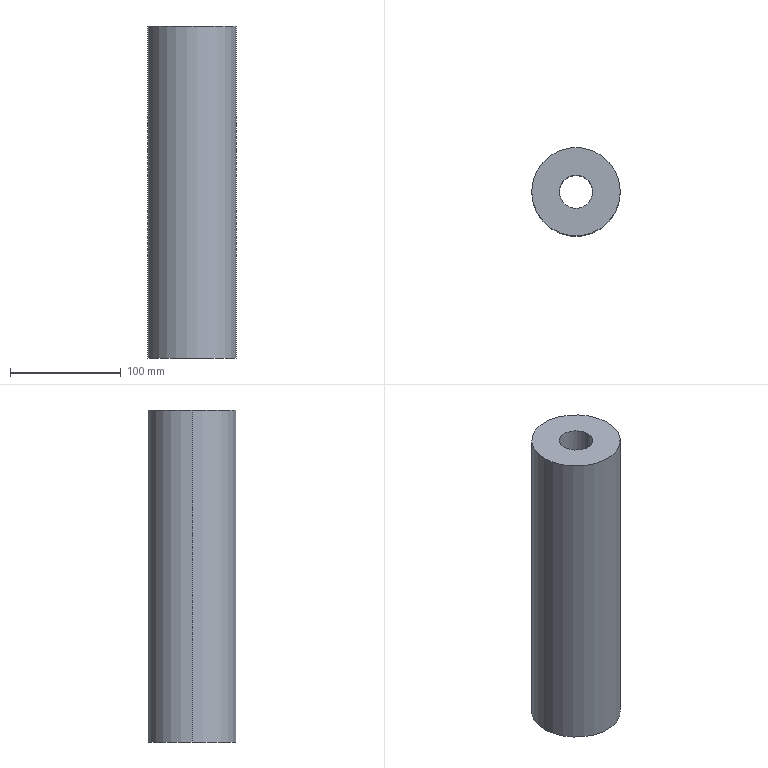Part | STEP file | Shaft for belt1V11 | 1 solid | 6 faces | box 80 x 80 x 300 mm | volume 1295907 mm3 | cylinder 4 | plane 2 | commonest cylinder face diameters 30 x2 80 x2
STEP:
#1=CARTESIAN_POINT('',(0.,0.,0.));
#2=DIRECTION('',(0.,0.,1.));
#3=DIRECTION('',(1.,0.,0.));
#4=AXIS2_PLACEMENT_3D('',#1,#2,#3);
#5=CARTESIAN_POINT('',(-15.,0.,300.));
#6=VERTEX_POINT('',#5);
#7=CARTESIAN_POINT('',(-15.,0.,0.));
#8=VERTEX_POINT('',#7);
#9=CARTESIAN_POINT('',(-15.,0.,300.));
#10=DIRECTION('',(0.,0.,-1.));
#11=VECTOR('',#10,1.);
#12=LINE('',#9,#11);
#13=CARTESIAN_POINT('',(0.,0.,300.));
#14=DIRECTION('',(0.,0.,-1.));
#15=DIRECTION('',(-1.,0.,0.));
#16=AXIS2_PLACEMENT_3D('',#13,#14,#15);
#17=CYLINDRICAL_SURFACE('',#16,15.);
#18=CARTESIAN_POINT('',(6.283,0.));
#19=DIRECTION('',(0.,1.));
#20=VECTOR('',#19,1.);
#21=LINE('',#18,#20);
#22=(GEOMETRIC_REPRESENTATION_CONTEXT(2)PARAMETRIC_REPRESENTATION_CONTEXT()REPRESENTATION_CONTEXT('',''));
#23=DEFINITIONAL_REPRESENTATION('',(#21),#22);
#24=PCURVE('',#17,#23);
#25=CARTESIAN_POINT('',(0.,0.,300.));
#26=DIRECTION('',(0.,0.,-1.));
#27=DIRECTION('',(-1.,0.,0.));
#28=AXIS2_PLACEMENT_3D('',#25,#26,#27);
#29=CYLINDRICAL_SURFACE('',#28,15.);
#30=CARTESIAN_POINT('',(0.,0.));
#31=DIRECTION('',(0.,1.));
#32=VECTOR('',#31,1.);
#33=LINE('',#30,#32);
#34=(GEOMETRIC_REPRESENTATION_CONTEXT(2)PARAMETRIC_REPRESENTATION_CONTEXT()REPRESENTATION_CONTEXT('',''));
#35=DEFINITIONAL_REPRESENTATION('',(#33),#34);
#36=PCURVE('',#29,#35);
#37=SURFACE_CURVE('',#12,(#24,#36),.PCURVE_S1.);
#38=EDGE_CURVE('',#6,#8,#37,.T.);
#39=ORIENTED_EDGE('',*,*,#38,.T.);
#40=CARTESIAN_POINT('',(15.,0.,0.));
#41=VERTEX_POINT('',#40);
#42=CARTESIAN_POINT('',(0.,0.,0.));
#43=DIRECTION('',(0.,0.,1.));
#44=DIRECTION('',(1.,0.,0.));
#45=AXIS2_PLACEMENT_3D('',#42,#43,#44);
#46=CIRCLE('',#45,15.);
#47=CARTESIAN_POINT('',(9.425,300.));
#48=DIRECTION('',(-1.,0.));
#49=VECTOR('',#48,1.);
#50=LINE('',#47,#49);
#51=(GEOMETRIC_REPRESENTATION_CONTEXT(2)PARAMETRIC_REPRESENTATION_CONTEXT()REPRESENTATION_CONTEXT('',''));
#52=DEFINITIONAL_REPRESENTATION('',(#50),#51);
#53=PCURVE('',#17,#52);
#54=CARTESIAN_POINT('',(0.,0.,0.));
#55=DIRECTION('',(0.,0.,1.));
#56=DIRECTION('',(1.,0.,0.));
#57=AXIS2_PLACEMENT_3D('',#54,#55,#56);
#58=PLANE('',#57);
#59=CARTESIAN_POINT('',(0.,0.));
#60=DIRECTION('',(1.,0.));
#61=AXIS2_PLACEMENT_2D('',#59,#60);
#62=CIRCLE('',#61,15.);
#63=(GEOMETRIC_REPRESENTATION_CONTEXT(2)PARAMETRIC_REPRESENTATION_CONTEXT()REPRESENTATION_CONTEXT('',''));
#64=DEFINITIONAL_REPRESENTATION('',(#62),#63);
#65=PCURVE('',#58,#64);
#66=SURFACE_CURVE('',#46,(#53,#65),.PCURVE_S1.);
#67=EDGE_CURVE('',#8,#41,#66,.T.);
#68=ORIENTED_EDGE('',*,*,#67,.T.);
#69=CARTESIAN_POINT('',(15.,0.,300.));
#70=VERTEX_POINT('',#69);
#71=CARTESIAN_POINT('',(15.,0.,300.));
#72=DIRECTION('',(0.,0.,-1.));
#73=VECTOR('',#72,1.);
#74=LINE('',#71,#73);
#75=CARTESIAN_POINT('',(3.142,0.));
#76=DIRECTION('',(0.,1.));
#77=VECTOR('',#76,1.);
#78=LINE('',#75,#77);
#79=(GEOMETRIC_REPRESENTATION_CONTEXT(2)PARAMETRIC_REPRESENTATION_CONTEXT()REPRESENTATION_CONTEXT('',''));
#80=DEFINITIONAL_REPRESENTATION('',(#78),#79);
#81=PCURVE('',#17,#80);
#82=CARTESIAN_POINT('',(3.142,0.));
#83=DIRECTION('',(0.,1.));
#84=VECTOR('',#83,1.);
#85=LINE('',#82,#84);
#86=(GEOMETRIC_REPRESENTATION_CONTEXT(2)PARAMETRIC_REPRESENTATION_CONTEXT()REPRESENTATION_CONTEXT('',''));
#87=DEFINITIONAL_REPRESENTATION('',(#85),#86);
#88=PCURVE('',#29,#87);
#89=SURFACE_CURVE('',#74,(#81,#88),.PCURVE_S1.);
#90=EDGE_CURVE('',#70,#41,#89,.T.);
#91=ORIENTED_EDGE('',*,*,#90,.F.);
#92=CARTESIAN_POINT('',(0.,0.,300.));
#93=DIRECTION('',(0.,0.,1.));
#94=DIRECTION('',(1.,0.,0.));
#95=AXIS2_PLACEMENT_3D('',#92,#93,#94);
#96=CIRCLE('',#95,15.);
#97=CARTESIAN_POINT('',(9.425,0.));
#98=DIRECTION('',(-1.,0.));
#99=VECTOR('',#98,1.);
#100=LINE('',#97,#99);
#101=(GEOMETRIC_REPRESENTATION_CONTEXT(2)PARAMETRIC_REPRESENTATION_CONTEXT()REPRESENTATION_CONTEXT('',''));
#102=DEFINITIONAL_REPRESENTATION('',(#100),#101);
#103=PCURVE('',#17,#102);
#104=CARTESIAN_POINT('',(0.,0.,300.));
#105=DIRECTION('',(0.,0.,1.));
#106=DIRECTION('',(1.,0.,0.));
#107=AXIS2_PLACEMENT_3D('',#104,#105,#106);
#108=PLANE('',#107);
#109=CARTESIAN_POINT('',(0.,0.));
#110=DIRECTION('',(1.,0.));
#111=AXIS2_PLACEMENT_2D('',#109,#110);
#112=CIRCLE('',#111,15.);
#113=(GEOMETRIC_REPRESENTATION_CONTEXT(2)PARAMETRIC_REPRESENTATION_CONTEXT()REPRESENTATION_CONTEXT('',''));
#114=DEFINITIONAL_REPRESENTATION('',(#112),#113);
#115=PCURVE('',#108,#114);
#116=SURFACE_CURVE('',#96,(#103,#115),.PCURVE_S1.);
#117=EDGE_CURVE('',#6,#70,#116,.T.);
#118=ORIENTED_EDGE('',*,*,#117,.F.);
#119=EDGE_LOOP('',(#39,#68,#91,#118));
#120=FACE_BOUND('',#119,.F.);
#121=ADVANCED_FACE('',(#120),#17,.F.);
#122=CARTESIAN_POINT('',(40.,0.,300.));
#123=VERTEX_POINT('',#122);
#124=CARTESIAN_POINT('',(-40.,0.,300.));
#125=VERTEX_POINT('',#124);
#126=CARTESIAN_POINT('',(0.,0.,300.));
#127=DIRECTION('',(0.,0.,1.));
#128=DIRECTION('',(1.,0.,0.));
#129=AXIS2_PLACEMENT_3D('',#126,#127,#128);
#130=CIRCLE('',#129,40.);
#131=CARTESIAN_POINT('',(0.,0.,300.));
#132=DIRECTION('',(0.,0.,-1.));
#133=DIRECTION('',(-1.,0.,0.));
#134=AXIS2_PLACEMENT_3D('',#131,#132,#133);
#135=CYLINDRICAL_SURFACE('',#134,40.);
#136=CARTESIAN_POINT('',(3.142,0.));
#137=DIRECTION('',(-1.,0.));
#138=VECTOR('',#137,1.);
#139=LINE('',#136,#138);
#140=(GEOMETRIC_REPRESENTATION_CONTEXT(2)PARAMETRIC_REPRESENTATION_CONTEXT()REPRESENTATION_CONTEXT('',''));
#141=DEFINITIONAL_REPRESENTATION('',(#139),#140);
#142=PCURVE('',#135,#141);
#143=CARTESIAN_POINT('',(0.,0.));
#144=DIRECTION('',(1.,0.));
#145=AXIS2_PLACEMENT_2D('',#143,#144);
#146=CIRCLE('',#145,40.);
#147=(GEOMETRIC_REPRESENTATION_CONTEXT(2)PARAMETRIC_REPRESENTATION_CONTEXT()REPRESENTATION_CONTEXT('',''));
#148=DEFINITIONAL_REPRESENTATION('',(#146),#147);
#149=PCURVE('',#108,#148);
#150=SURFACE_CURVE('',#130,(#142,#149),.PCURVE_S1.);
#151=EDGE_CURVE('',#123,#125,#150,.T.);
#152=ORIENTED_EDGE('',*,*,#151,.F.);
#153=CARTESIAN_POINT('',(40.,0.,0.));
#154=VERTEX_POINT('',#153);
#155=CARTESIAN_POINT('',(40.,0.,300.));
#156=DIRECTION('',(0.,0.,-1.));
#157=VECTOR('',#156,1.);
#158=LINE('',#155,#157);
#159=CARTESIAN_POINT('',(3.142,0.));
#160=DIRECTION('',(0.,1.));
#161=VECTOR('',#160,1.);
#162=LINE('',#159,#161);
#163=(GEOMETRIC_REPRESENTATION_CONTEXT(2)PARAMETRIC_REPRESENTATION_CONTEXT()REPRESENTATION_CONTEXT('',''));
#164=DEFINITIONAL_REPRESENTATION('',(#162),#163);
#165=PCURVE('',#135,#164);
#166=CARTESIAN_POINT('',(0.,0.,300.));
#167=DIRECTION('',(0.,0.,-1.));
#168=DIRECTION('',(-1.,0.,0.));
#169=AXIS2_PLACEMENT_3D('',#166,#167,#168);
#170=CYLINDRICAL_SURFACE('',#169,40.);
#171=CARTESIAN_POINT('',(3.142,0.));
#172=DIRECTION('',(0.,1.));
#173=VECTOR('',#172,1.);
#174=LINE('',#171,#173);
#175=(GEOMETRIC_REPRESENTATION_CONTEXT(2)PARAMETRIC_REPRESENTATION_CONTEXT()REPRESENTATION_CONTEXT('',''));
#176=DEFINITIONAL_REPRESENTATION('',(#174),#175);
#177=PCURVE('',#170,#176);
#178=SURFACE_CURVE('',#158,(#165,#177),.PCURVE_S1.);
#179=EDGE_CURVE('',#123,#154,#178,.T.);
#180=ORIENTED_EDGE('',*,*,#179,.T.);
#181=CARTESIAN_POINT('',(-40.,0.,0.));
#182=VERTEX_POINT('',#181);
#183=CARTESIAN_POINT('',(0.,0.,0.));
#184=DIRECTION('',(0.,0.,1.));
#185=DIRECTION('',(1.,0.,0.));
#186=AXIS2_PLACEMENT_3D('',#183,#184,#185);
#187=CIRCLE('',#186,40.);
#188=CARTESIAN_POINT('',(3.142,300.));
#189=DIRECTION('',(-1.,0.));
#190=VECTOR('',#189,1.);
#191=LINE('',#188,#190);
#192=(GEOMETRIC_REPRESENTATION_CONTEXT(2)PARAMETRIC_REPRESENTATION_CONTEXT()REPRESENTATION_CONTEXT('',''));
#193=DEFINITIONAL_REPRESENTATION('',(#191),#192);
#194=PCURVE('',#135,#193);
#195=CARTESIAN_POINT('',(0.,0.));
#196=DIRECTION('',(1.,0.));
#197=AXIS2_PLACEMENT_2D('',#195,#196);
#198=CIRCLE('',#197,40.);
#199=(GEOMETRIC_REPRESENTATION_CONTEXT(2)PARAMETRIC_REPRESENTATION_CONTEXT()REPRESENTATION_CONTEXT('',''));
#200=DEFINITIONAL_REPRESENTATION('',(#198),#199);
#201=PCURVE('',#58,#200);
#202=SURFACE_CURVE('',#187,(#194,#201),.PCURVE_S1.);
#203=EDGE_CURVE('',#154,#182,#202,.T.);
#204=ORIENTED_EDGE('',*,*,#203,.T.);
#205=CARTESIAN_POINT('',(-40.,0.,300.));
#206=DIRECTION('',(0.,0.,-1.));
#207=VECTOR('',#206,1.);
#208=LINE('',#205,#207);
#209=CARTESIAN_POINT('',(0.,0.));
#210=DIRECTION('',(0.,1.));
#211=VECTOR('',#210,1.);
#212=LINE('',#209,#211);
#213=(GEOMETRIC_REPRESENTATION_CONTEXT(2)PARAMETRIC_REPRESENTATION_CONTEXT()REPRESENTATION_CONTEXT('',''));
#214=DEFINITIONAL_REPRESENTATION('',(#212),#213);
#215=PCURVE('',#135,#214);
#216=CARTESIAN_POINT('',(6.283,0.));
#217=DIRECTION('',(0.,1.));
#218=VECTOR('',#217,1.);
#219=LINE('',#216,#218);
#220=(GEOMETRIC_REPRESENTATION_CONTEXT(2)PARAMETRIC_REPRESENTATION_CONTEXT()REPRESENTATION_CONTEXT('',''));
#221=DEFINITIONAL_REPRESENTATION('',(#219),#220);
#222=PCURVE('',#170,#221);
#223=SURFACE_CURVE('',#208,(#215,#222),.PCURVE_S1.);
#224=EDGE_CURVE('',#125,#182,#223,.T.);
#225=ORIENTED_EDGE('',*,*,#224,.F.);
#226=EDGE_LOOP('',(#152,#180,#204,#225));
#227=FACE_BOUND('',#226,.T.);
#228=ADVANCED_FACE('',(#227),#135,.T.);
#229=CARTESIAN_POINT('',(0.,0.,300.));
#230=DIRECTION('',(0.,0.,1.));
#231=DIRECTION('',(1.,0.,0.));
#232=AXIS2_PLACEMENT_3D('',#229,#230,#231);
#233=CIRCLE('',#232,40.);
#234=CARTESIAN_POINT('',(0.,0.));
#235=DIRECTION('',(1.,0.));
#236=AXIS2_PLACEMENT_2D('',#234,#235);
#237=CIRCLE('',#236,40.);
#238=(GEOMETRIC_REPRESENTATION_CONTEXT(2)PARAMETRIC_REPRESENTATION_CONTEXT()REPRESENTATION_CONTEXT('',''));
#239=DEFINITIONAL_REPRESENTATION('',(#237),#238);
#240=PCURVE('',#108,#239);
#241=CARTESIAN_POINT('',(9.425,0.));
#242=DIRECTION('',(-1.,0.));
#243=VECTOR('',#242,1.);
#244=LINE('',#241,#243);
#245=(GEOMETRIC_REPRESENTATION_CONTEXT(2)PARAMETRIC_REPRESENTATION_CONTEXT()REPRESENTATION_CONTEXT('',''));
#246=DEFINITIONAL_REPRESENTATION('',(#244),#245);
#247=PCURVE('',#170,#246);
#248=SURFACE_CURVE('',#233,(#240,#247),.PCURVE_S1.);
#249=EDGE_CURVE('',#125,#123,#248,.T.);
#250=ORIENTED_EDGE('',*,*,#249,.T.);
#251=ORIENTED_EDGE('',*,*,#151,.T.);
#252=EDGE_LOOP('',(#250,#251));
#253=FACE_BOUND('',#252,.T.);
#254=ORIENTED_EDGE('',*,*,#117,.F.);
#255=CARTESIAN_POINT('',(0.,0.,300.));
#256=DIRECTION('',(0.,0.,1.));
#257=DIRECTION('',(1.,0.,0.));
#258=AXIS2_PLACEMENT_3D('',#255,#256,#257);
#259=CIRCLE('',#258,15.);
#260=CARTESIAN_POINT('',(0.,0.));
#261=DIRECTION('',(1.,0.));
#262=AXIS2_PLACEMENT_2D('',#260,#261);
#263=CIRCLE('',#262,15.);
#264=(GEOMETRIC_REPRESENTATION_CONTEXT(2)PARAMETRIC_REPRESENTATION_CONTEXT()REPRESENTATION_CONTEXT('',''));
#265=DEFINITIONAL_REPRESENTATION('',(#263),#264);
#266=PCURVE('',#108,#265);
#267=CARTESIAN_POINT('',(3.142,0.));
#268=DIRECTION('',(-1.,0.));
#269=VECTOR('',#268,1.);
#270=LINE('',#267,#269);
#271=(GEOMETRIC_REPRESENTATION_CONTEXT(2)PARAMETRIC_REPRESENTATION_CONTEXT()REPRESENTATION_CONTEXT('',''));
#272=DEFINITIONAL_REPRESENTATION('',(#270),#271);
#273=PCURVE('',#29,#272);
#274=SURFACE_CURVE('',#259,(#266,#273),.PCURVE_S1.);
#275=EDGE_CURVE('',#70,#6,#274,.T.);
#276=ORIENTED_EDGE('',*,*,#275,.F.);
#277=EDGE_LOOP('',(#254,#276));
#278=FACE_BOUND('',#277,.T.);
#279=ADVANCED_FACE('',(#253,#278),#108,.T.);
#280=CARTESIAN_POINT('',(0.,0.,0.));
#281=DIRECTION('',(0.,0.,1.));
#282=DIRECTION('',(1.,0.,0.));
#283=AXIS2_PLACEMENT_3D('',#280,#281,#282);
#284=CIRCLE('',#283,40.);
#285=CARTESIAN_POINT('',(0.,0.));
#286=DIRECTION('',(1.,0.));
#287=AXIS2_PLACEMENT_2D('',#285,#286);
#288=CIRCLE('',#287,40.);
#289=(GEOMETRIC_REPRESENTATION_CONTEXT(2)PARAMETRIC_REPRESENTATION_CONTEXT()REPRESENTATION_CONTEXT('',''));
#290=DEFINITIONAL_REPRESENTATION('',(#288),#289);
#291=PCURVE('',#58,#290);
#292=CARTESIAN_POINT('',(9.425,300.));
#293=DIRECTION('',(-1.,0.));
#294=VECTOR('',#293,1.);
#295=LINE('',#292,#294);
#296=(GEOMETRIC_REPRESENTATION_CONTEXT(2)PARAMETRIC_REPRESENTATION_CONTEXT()REPRESENTATION_CONTEXT('',''));
#297=DEFINITIONAL_REPRESENTATION('',(#295),#296);
#298=PCURVE('',#170,#297);
#299=SURFACE_CURVE('',#284,(#291,#298),.PCURVE_S1.);
#300=EDGE_CURVE('',#182,#154,#299,.T.);
#301=ORIENTED_EDGE('',*,*,#300,.F.);
#302=ORIENTED_EDGE('',*,*,#203,.F.);
#303=EDGE_LOOP('',(#301,#302));
#304=FACE_BOUND('',#303,.T.);
#305=ORIENTED_EDGE('',*,*,#67,.T.);
#306=CARTESIAN_POINT('',(0.,0.,0.));
#307=DIRECTION('',(0.,0.,1.));
#308=DIRECTION('',(1.,0.,0.));
#309=AXIS2_PLACEMENT_3D('',#306,#307,#308);
#310=CIRCLE('',#309,15.);
#311=CARTESIAN_POINT('',(0.,0.));
#312=DIRECTION('',(1.,0.));
#313=AXIS2_PLACEMENT_2D('',#311,#312);
#314=CIRCLE('',#313,15.);
#315=(GEOMETRIC_REPRESENTATION_CONTEXT(2)PARAMETRIC_REPRESENTATION_CONTEXT()REPRESENTATION_CONTEXT('',''));
#316=DEFINITIONAL_REPRESENTATION('',(#314),#315);
#317=PCURVE('',#58,#316);
#318=CARTESIAN_POINT('',(3.142,300.));
#319=DIRECTION('',(-1.,0.));
#320=VECTOR('',#319,1.);
#321=LINE('',#318,#320);
#322=(GEOMETRIC_REPRESENTATION_CONTEXT(2)PARAMETRIC_REPRESENTATION_CONTEXT()REPRESENTATION_CONTEXT('',''));
#323=DEFINITIONAL_REPRESENTATION('',(#321),#322);
#324=PCURVE('',#29,#323);
#325=SURFACE_CURVE('',#310,(#317,#324),.PCURVE_S1.);
#326=EDGE_CURVE('',#41,#8,#325,.T.);
#327=ORIENTED_EDGE('',*,*,#326,.T.);
#328=EDGE_LOOP('',(#305,#327));
#329=FACE_BOUND('',#328,.T.);
#330=ADVANCED_FACE('',(#304,#329),#58,.F.);
#331=ORIENTED_EDGE('',*,*,#179,.F.);
#332=ORIENTED_EDGE('',*,*,#249,.F.);
#333=ORIENTED_EDGE('',*,*,#224,.T.);
#334=ORIENTED_EDGE('',*,*,#300,.T.);
#335=EDGE_LOOP('',(#331,#332,#333,#334));
#336=FACE_BOUND('',#335,.T.);
#337=ADVANCED_FACE('',(#336),#170,.T.);
#338=ORIENTED_EDGE('',*,*,#326,.T.);
#339=ORIENTED_EDGE('',*,*,#38,.F.);
#340=ORIENTED_EDGE('',*,*,#275,.F.);
#341=ORIENTED_EDGE('',*,*,#90,.T.);
#342=EDGE_LOOP('',(#338,#339,#340,#341));
#343=FACE_BOUND('',#342,.F.);
#344=ADVANCED_FACE('',(#343),#29,.F.);
#345=CLOSED_SHELL('',(#121,#228,#279,#330,#337,#344));
#346=MANIFOLD_SOLID_BREP('',#345);
#347=(LENGTH_UNIT()NAMED_UNIT(*)SI_UNIT(.MILLI.,.METRE.));
#348=UNCERTAINTY_MEASURE_WITH_UNIT(LENGTH_MEASURE(0.0000001),#347,'','');
#349=(NAMED_UNIT(*)PLANE_ANGLE_UNIT()SI_UNIT($,.RADIAN.));
#350=(NAMED_UNIT(*)SI_UNIT($,.STERADIAN.)SOLID_ANGLE_UNIT());
#351=(GEOMETRIC_REPRESENTATION_CONTEXT(3)GLOBAL_UNCERTAINTY_ASSIGNED_CONTEXT((#348))GLOBAL_UNIT_ASSIGNED_CONTEXT((#347,#349,#350))REPRESENTATION_CONTEXT('',''));
#352=ADVANCED_BREP_SHAPE_REPRESENTATION('',(#4,#346),#351);